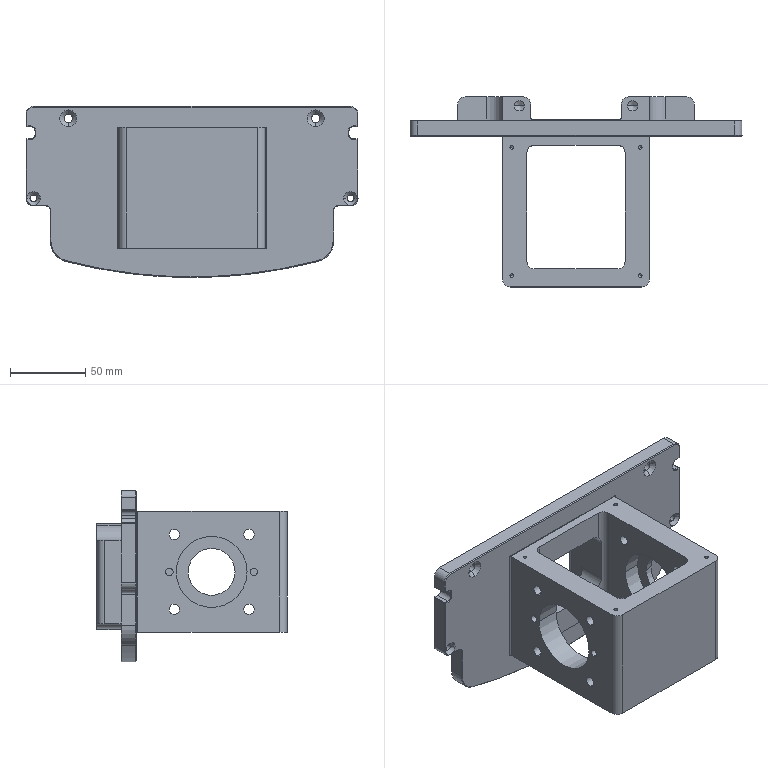Part | SolidWorks | features BaseBody 1 | 1 solid | 228 faces | box 220 x 126 x 113.5 mm | volume 568343 mm3 | cylinder 110 | plane 65 | cone 53 | commonest cylinder face diameters 6.8 x20 10 x20 2.5 x16 5 x8 2 x6 6 x6